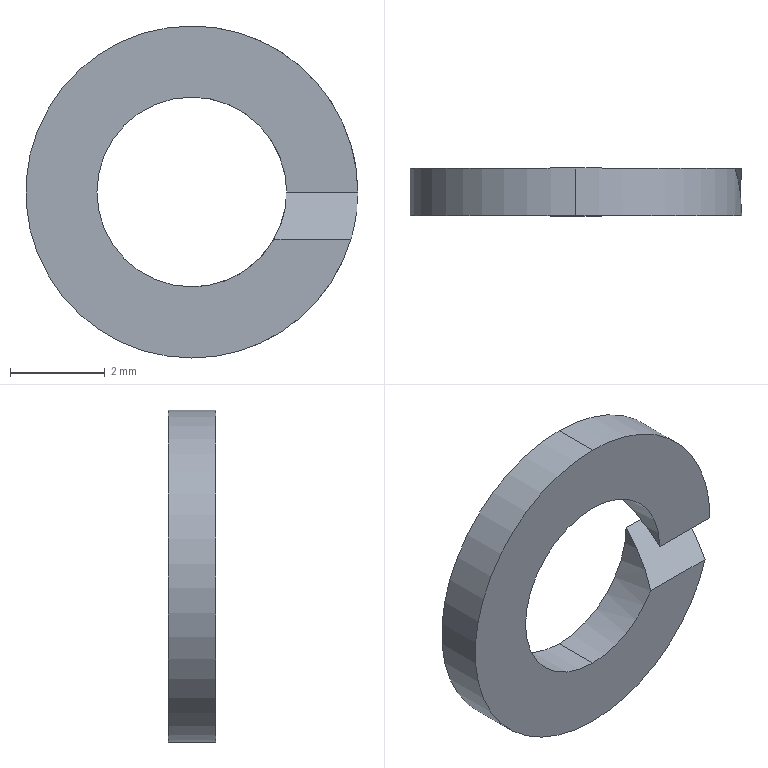Part | SolidWorks | features BaseBody 1 | 1 solid | 10 faces | box 7 x 1 x 7 mm | volume 24.399 mm3 | cylinder 6 | plane 4 | commonest cylinder face diameters 4 x3 7 x3
STEP:
#1=CARTESIAN_POINT('',(-17.5,26.,-23.5));
#2=VERTEX_POINT('',#1);
#3=CARTESIAN_POINT('',(-14.146,26.,-21.));
#4=VERTEX_POINT('',#3);
#5=CARTESIAN_POINT('',(-17.5,26.,-20.));
#6=DIRECTION('',(0.,-1.,0.));
#7=DIRECTION('',(0.,0.,1.));
#8=AXIS2_PLACEMENT_3D('',#5,#6,#7);
#9=CIRCLE('',#8,3.5);
#10=EDGE_CURVE('',#2,#4,#9,.T.);
#11=ORIENTED_EDGE('',*,*,#10,.F.);
#12=CARTESIAN_POINT('',(-17.5,27.,-23.5));
#13=VERTEX_POINT('',#12);
#14=CARTESIAN_POINT('',(-17.5,26.5,-23.5));
#15=DIRECTION('',(0.,1.,0.));
#16=VECTOR('',#15,1000.);
#17=LINE('',#14,#16);
#18=EDGE_CURVE('',#2,#13,#17,.T.);
#19=ORIENTED_EDGE('',*,*,#18,.T.);
#20=CARTESIAN_POINT('',(-14.,27.,-20.));
#21=VERTEX_POINT('',#20);
#22=CARTESIAN_POINT('',(-17.5,27.,-20.));
#23=DIRECTION('',(0.,-1.,0.));
#24=DIRECTION('',(0.,0.,1.));
#25=AXIS2_PLACEMENT_3D('',#22,#23,#24);
#26=CIRCLE('',#25,3.5);
#27=EDGE_CURVE('',#13,#21,#26,.T.);
#28=ORIENTED_EDGE('',*,*,#27,.T.);
#29=CARTESIAN_POINT('',(-14.,27.,-20.));
#30=CARTESIAN_POINT('',(-14.,26.661,-20.339));
#31=CARTESIAN_POINT('',(-14.049,26.325,-20.675));
#32=CARTESIAN_POINT('',(-14.146,26.,-21.));
#33=(BOUNDED_CURVE()B_SPLINE_CURVE(3,(#29,#30,#31,#32),.UNSPECIFIED.,.F.,.F.)B_SPLINE_CURVE_WITH_KNOTS((4,4),(1.571,1.861),.UNSPECIFIED.)CURVE()GEOMETRIC_REPRESENTATION_ITEM()RATIONAL_B_SPLINE_CURVE((1.,0.993,0.993,1.))REPRESENTATION_ITEM(''));
#34=EDGE_CURVE('',#21,#4,#33,.T.);
#35=ORIENTED_EDGE('',*,*,#34,.T.);
#36=EDGE_LOOP('',(#11,#19,#28,#35));
#37=FACE_OUTER_BOUND('',#36,.T.);
#38=CARTESIAN_POINT('',(-17.5,26.5,-20.));
#39=DIRECTION('',(0.,1.,0.));
#40=DIRECTION('',(0.,0.,1.));
#41=AXIS2_PLACEMENT_3D('',#38,#39,#40);
#42=CYLINDRICAL_SURFACE('',#41,3.5);
#43=ADVANCED_FACE('',(#37),#42,.T.);
#44=ORIENTED_EDGE('',*,*,#18,.F.);
#45=CARTESIAN_POINT('',(-17.5,26.,-16.5));
#46=VERTEX_POINT('',#45);
#47=CARTESIAN_POINT('',(-17.5,26.,-20.));
#48=DIRECTION('',(0.,-1.,0.));
#49=DIRECTION('',(0.,0.,1.));
#50=AXIS2_PLACEMENT_3D('',#47,#48,#49);
#51=CIRCLE('',#50,3.5);
#52=EDGE_CURVE('',#46,#2,#51,.T.);
#53=ORIENTED_EDGE('',*,*,#52,.F.);
#54=CARTESIAN_POINT('',(-17.5,27.,-16.5));
#55=VERTEX_POINT('',#54);
#56=CARTESIAN_POINT('',(-17.5,26.5,-16.5));
#57=DIRECTION('',(0.,1.,0.));
#58=VECTOR('',#57,1000.);
#59=LINE('',#56,#58);
#60=EDGE_CURVE('',#46,#55,#59,.T.);
#61=ORIENTED_EDGE('',*,*,#60,.T.);
#62=CARTESIAN_POINT('',(-17.5,27.,-20.));
#63=DIRECTION('',(0.,-1.,0.));
#64=DIRECTION('',(0.,0.,1.));
#65=AXIS2_PLACEMENT_3D('',#62,#63,#64);
#66=CIRCLE('',#65,3.5);
#67=EDGE_CURVE('',#55,#13,#66,.T.);
#68=ORIENTED_EDGE('',*,*,#67,.T.);
#69=EDGE_LOOP('',(#44,#53,#61,#68));
#70=FACE_OUTER_BOUND('',#69,.T.);
#71=CARTESIAN_POINT('',(-17.5,26.5,-20.));
#72=DIRECTION('',(0.,1.,0.));
#73=DIRECTION('',(0.,0.,1.));
#74=AXIS2_PLACEMENT_3D('',#71,#72,#73);
#75=CYLINDRICAL_SURFACE('',#74,3.5);
#76=ADVANCED_FACE('',(#70),#75,.T.);
#77=CARTESIAN_POINT('',(-17.5,26.,-22.));
#78=VERTEX_POINT('',#77);
#79=CARTESIAN_POINT('',(-17.5,26.,-18.));
#80=VERTEX_POINT('',#79);
#81=CARTESIAN_POINT('',(-17.5,26.,-20.));
#82=DIRECTION('',(0.,1.,0.));
#83=DIRECTION('',(0.,0.,1.));
#84=AXIS2_PLACEMENT_3D('',#81,#82,#83);
#85=CIRCLE('',#84,2.);
#86=EDGE_CURVE('',#78,#80,#85,.T.);
#87=ORIENTED_EDGE('',*,*,#86,.F.);
#88=CARTESIAN_POINT('',(-17.5,27.,-22.));
#89=VERTEX_POINT('',#88);
#90=CARTESIAN_POINT('',(-17.5,26.5,-22.));
#91=DIRECTION('',(0.,1.,0.));
#92=VECTOR('',#91,1000.);
#93=LINE('',#90,#92);
#94=EDGE_CURVE('',#78,#89,#93,.T.);
#95=ORIENTED_EDGE('',*,*,#94,.T.);
#96=CARTESIAN_POINT('',(-17.5,27.,-18.));
#97=VERTEX_POINT('',#96);
#98=CARTESIAN_POINT('',(-17.5,27.,-20.));
#99=DIRECTION('',(0.,-1.,0.));
#100=DIRECTION('',(0.,0.,1.));
#101=AXIS2_PLACEMENT_3D('',#98,#99,#100);
#102=CIRCLE('',#101,2.);
#103=EDGE_CURVE('',#97,#89,#102,.T.);
#104=ORIENTED_EDGE('',*,*,#103,.F.);
#105=CARTESIAN_POINT('',(-17.5,26.5,-18.));
#106=DIRECTION('',(0.,1.,0.));
#107=VECTOR('',#106,1000.);
#108=LINE('',#105,#107);
#109=EDGE_CURVE('',#80,#97,#108,.T.);
#110=ORIENTED_EDGE('',*,*,#109,.F.);
#111=EDGE_LOOP('',(#87,#95,#104,#110));
#112=FACE_OUTER_BOUND('',#111,.T.);
#113=CARTESIAN_POINT('',(-17.5,26.5,-20.));
#114=DIRECTION('',(0.,1.,0.));
#115=DIRECTION('',(0.,0.,1.));
#116=AXIS2_PLACEMENT_3D('',#113,#114,#115);
#117=CYLINDRICAL_SURFACE('',#116,2.);
#118=ADVANCED_FACE('',(#112),#117,.F.);
#119=CARTESIAN_POINT('',(-15.5,26.,-20.));
#120=VERTEX_POINT('',#119);
#121=CARTESIAN_POINT('',(-17.5,26.,-20.));
#122=DIRECTION('',(0.,1.,0.));
#123=DIRECTION('',(0.,0.,1.));
#124=AXIS2_PLACEMENT_3D('',#121,#122,#123);
#125=CIRCLE('',#124,2.);
#126=EDGE_CURVE('',#80,#120,#125,.T.);
#127=ORIENTED_EDGE('',*,*,#126,.F.);
#128=ORIENTED_EDGE('',*,*,#109,.T.);
#129=CARTESIAN_POINT('',(-15.768,27.,-19.));
#130=VERTEX_POINT('',#129);
#131=CARTESIAN_POINT('',(-17.5,27.,-20.));
#132=DIRECTION('',(0.,-1.,0.));
#133=DIRECTION('',(0.,0.,1.));
#134=AXIS2_PLACEMENT_3D('',#131,#132,#133);
#135=CIRCLE('',#134,2.);
#136=EDGE_CURVE('',#130,#97,#135,.T.);
#137=ORIENTED_EDGE('',*,*,#136,.F.);
#138=CARTESIAN_POINT('',(-15.768,27.,-19.));
#139=CARTESIAN_POINT('',(-15.591,26.694,-19.306));
#140=CARTESIAN_POINT('',(-15.5,26.353,-19.647));
#141=CARTESIAN_POINT('',(-15.5,26.,-20.));
#142=(BOUNDED_CURVE()B_SPLINE_CURVE(3,(#138,#139,#140,#141),.UNSPECIFIED.,.F.,.F.)B_SPLINE_CURVE_WITH_KNOTS((4,4),(1.047,1.571),.UNSPECIFIED.)CURVE()GEOMETRIC_REPRESENTATION_ITEM()RATIONAL_B_SPLINE_CURVE((1.,0.9773,0.9773,1.))REPRESENTATION_ITEM(''));
#143=EDGE_CURVE('',#130,#120,#142,.T.);
#144=ORIENTED_EDGE('',*,*,#143,.T.);
#145=EDGE_LOOP('',(#127,#128,#137,#144));
#146=FACE_OUTER_BOUND('',#145,.T.);
#147=CARTESIAN_POINT('',(-17.5,26.5,-20.));
#148=DIRECTION('',(0.,1.,0.));
#149=DIRECTION('',(0.,0.,1.));
#150=AXIS2_PLACEMENT_3D('',#147,#148,#149);
#151=CYLINDRICAL_SURFACE('',#150,2.);
#152=ADVANCED_FACE('',(#146),#151,.F.);
#153=CARTESIAN_POINT('',(-14.146,27.,-19.));
#154=VERTEX_POINT('',#153);
#155=CARTESIAN_POINT('',(-17.5,27.,-19.));
#156=DIRECTION('',(-1.,0.,0.));
#157=VECTOR('',#156,1000.);
#158=LINE('',#155,#157);
#159=EDGE_CURVE('',#154,#130,#158,.T.);
#160=ORIENTED_EDGE('',*,*,#159,.T.);
#161=ORIENTED_EDGE('',*,*,#136,.T.);
#162=ORIENTED_EDGE('',*,*,#103,.T.);
#163=CARTESIAN_POINT('',(-15.5,27.,-20.));
#164=VERTEX_POINT('',#163);
#165=CARTESIAN_POINT('',(-17.5,27.,-20.));
#166=DIRECTION('',(0.,-1.,0.));
#167=DIRECTION('',(0.,0.,1.));
#168=AXIS2_PLACEMENT_3D('',#165,#166,#167);
#169=CIRCLE('',#168,2.);
#170=EDGE_CURVE('',#89,#164,#169,.T.);
#171=ORIENTED_EDGE('',*,*,#170,.T.);
#172=CARTESIAN_POINT('',(-17.5,27.,-20.));
#173=DIRECTION('',(1.,0.,0.));
#174=VECTOR('',#173,1000.);
#175=LINE('',#172,#174);
#176=EDGE_CURVE('',#164,#21,#175,.T.);
#177=ORIENTED_EDGE('',*,*,#176,.T.);
#178=ORIENTED_EDGE('',*,*,#27,.F.);
#179=ORIENTED_EDGE('',*,*,#67,.F.);
#180=CARTESIAN_POINT('',(-17.5,27.,-20.));
#181=DIRECTION('',(0.,-1.,0.));
#182=DIRECTION('',(0.,0.,1.));
#183=AXIS2_PLACEMENT_3D('',#180,#181,#182);
#184=CIRCLE('',#183,3.5);
#185=EDGE_CURVE('',#154,#55,#184,.T.);
#186=ORIENTED_EDGE('',*,*,#185,.F.);
#187=EDGE_LOOP('',(#160,#161,#162,#171,#177,#178,#179,#186));
#188=FACE_OUTER_BOUND('',#187,.T.);
#189=CARTESIAN_POINT('',(-17.5,27.,-17.25));
#190=DIRECTION('',(0.,1.,0.));
#191=DIRECTION('',(1.,0.,0.));
#192=AXIS2_PLACEMENT_3D('',#189,#190,#191);
#193=PLANE('',#192);
#194=ADVANCED_FACE('',(#188),#193,.T.);
#195=CARTESIAN_POINT('',(-15.768,26.,-21.));
#196=VERTEX_POINT('',#195);
#197=CARTESIAN_POINT('',(-17.5,26.,-21.));
#198=DIRECTION('',(-1.,0.,0.));
#199=VECTOR('',#198,1000.);
#200=LINE('',#197,#199);
#201=EDGE_CURVE('',#4,#196,#200,.T.);
#202=ORIENTED_EDGE('',*,*,#201,.F.);
#203=ORIENTED_EDGE('',*,*,#34,.F.);
#204=ORIENTED_EDGE('',*,*,#176,.F.);
#205=CARTESIAN_POINT('',(-15.5,27.,-20.));
#206=CARTESIAN_POINT('',(-15.5,26.647,-20.353));
#207=CARTESIAN_POINT('',(-15.591,26.306,-20.694));
#208=CARTESIAN_POINT('',(-15.768,26.,-21.));
#209=(BOUNDED_CURVE()B_SPLINE_CURVE(3,(#205,#206,#207,#208),.UNSPECIFIED.,.F.,.F.)B_SPLINE_CURVE_WITH_KNOTS((4,4),(1.571,2.094),.UNSPECIFIED.)CURVE()GEOMETRIC_REPRESENTATION_ITEM()RATIONAL_B_SPLINE_CURVE((1.,0.9773,0.9773,1.))REPRESENTATION_ITEM(''));
#210=EDGE_CURVE('',#164,#196,#209,.T.);
#211=ORIENTED_EDGE('',*,*,#210,.T.);
#212=EDGE_LOOP('',(#202,#203,#204,#211));
#213=FACE_OUTER_BOUND('',#212,.T.);
#214=CARTESIAN_POINT('',(-17.5,27.,-20.));
#215=DIRECTION('',(0.,0.7071,-0.7071));
#216=DIRECTION('',(-1.,0.,0.));
#217=AXIS2_PLACEMENT_3D('',#214,#215,#216);
#218=PLANE('',#217);
#219=ADVANCED_FACE('',(#213),#218,.F.);
#220=ORIENTED_EDGE('',*,*,#159,.F.);
#221=CARTESIAN_POINT('',(-14.,26.,-20.));
#222=VERTEX_POINT('',#221);
#223=CARTESIAN_POINT('',(-14.,26.,-20.));
#224=CARTESIAN_POINT('',(-14.,26.339,-19.661));
#225=CARTESIAN_POINT('',(-14.049,26.675,-19.325));
#226=CARTESIAN_POINT('',(-14.146,27.,-19.));
#227=(BOUNDED_CURVE()B_SPLINE_CURVE(3,(#223,#224,#225,#226),.UNSPECIFIED.,.F.,.T.)B_SPLINE_CURVE_WITH_KNOTS((4,4),(4.712,5.002),.UNSPECIFIED.)CURVE()GEOMETRIC_REPRESENTATION_ITEM()RATIONAL_B_SPLINE_CURVE((1.,0.993,0.993,1.))REPRESENTATION_ITEM(''));
#228=EDGE_CURVE('',#222,#154,#227,.T.);
#229=ORIENTED_EDGE('',*,*,#228,.F.);
#230=CARTESIAN_POINT('',(-17.5,26.,-20.));
#231=DIRECTION('',(1.,0.,0.));
#232=VECTOR('',#231,1000.);
#233=LINE('',#230,#232);
#234=EDGE_CURVE('',#120,#222,#233,.T.);
#235=ORIENTED_EDGE('',*,*,#234,.F.);
#236=ORIENTED_EDGE('',*,*,#143,.F.);
#237=EDGE_LOOP('',(#220,#229,#235,#236));
#238=FACE_OUTER_BOUND('',#237,.T.);
#239=CARTESIAN_POINT('',(-17.5,26.,-20.));
#240=DIRECTION('',(0.,-0.7071,0.7071));
#241=DIRECTION('',(-1.,0.,0.));
#242=AXIS2_PLACEMENT_3D('',#239,#240,#241);
#243=PLANE('',#242);
#244=ADVANCED_FACE('',(#238),#243,.F.);
#245=ORIENTED_EDGE('',*,*,#234,.T.);
#246=CARTESIAN_POINT('',(-17.5,26.,-20.));
#247=DIRECTION('',(0.,-1.,0.));
#248=DIRECTION('',(0.,0.,1.));
#249=AXIS2_PLACEMENT_3D('',#246,#247,#248);
#250=CIRCLE('',#249,3.5);
#251=EDGE_CURVE('',#222,#46,#250,.T.);
#252=ORIENTED_EDGE('',*,*,#251,.T.);
#253=ORIENTED_EDGE('',*,*,#52,.T.);
#254=ORIENTED_EDGE('',*,*,#10,.T.);
#255=ORIENTED_EDGE('',*,*,#201,.T.);
#256=CARTESIAN_POINT('',(-17.5,26.,-20.));
#257=DIRECTION('',(0.,1.,0.));
#258=DIRECTION('',(0.,0.,1.));
#259=AXIS2_PLACEMENT_3D('',#256,#257,#258);
#260=CIRCLE('',#259,2.);
#261=EDGE_CURVE('',#196,#78,#260,.T.);
#262=ORIENTED_EDGE('',*,*,#261,.T.);
#263=ORIENTED_EDGE('',*,*,#86,.T.);
#264=ORIENTED_EDGE('',*,*,#126,.T.);
#265=EDGE_LOOP('',(#245,#252,#253,#254,#255,#262,#263,#264));
#266=FACE_OUTER_BOUND('',#265,.T.);
#267=CARTESIAN_POINT('',(-17.5,26.,-17.25));
#268=DIRECTION('',(0.,-1.,0.));
#269=DIRECTION('',(0.,0.,-1.));
#270=AXIS2_PLACEMENT_3D('',#267,#268,#269);
#271=PLANE('',#270);
#272=ADVANCED_FACE('',(#266),#271,.T.);
#273=ORIENTED_EDGE('',*,*,#94,.F.);
#274=ORIENTED_EDGE('',*,*,#261,.F.);
#275=ORIENTED_EDGE('',*,*,#210,.F.);
#276=ORIENTED_EDGE('',*,*,#170,.F.);
#277=EDGE_LOOP('',(#273,#274,#275,#276));
#278=FACE_OUTER_BOUND('',#277,.T.);
#279=CARTESIAN_POINT('',(-17.5,26.5,-20.));
#280=DIRECTION('',(0.,1.,0.));
#281=DIRECTION('',(0.,0.,1.));
#282=AXIS2_PLACEMENT_3D('',#279,#280,#281);
#283=CYLINDRICAL_SURFACE('',#282,2.);
#284=ADVANCED_FACE('',(#278),#283,.F.);
#285=ORIENTED_EDGE('',*,*,#60,.F.);
#286=ORIENTED_EDGE('',*,*,#251,.F.);
#287=ORIENTED_EDGE('',*,*,#228,.T.);
#288=ORIENTED_EDGE('',*,*,#185,.T.);
#289=EDGE_LOOP('',(#285,#286,#287,#288));
#290=FACE_OUTER_BOUND('',#289,.T.);
#291=CARTESIAN_POINT('',(-17.5,26.5,-20.));
#292=DIRECTION('',(0.,1.,0.));
#293=DIRECTION('',(0.,0.,1.));
#294=AXIS2_PLACEMENT_3D('',#291,#292,#293);
#295=CYLINDRICAL_SURFACE('',#294,3.5);
#296=ADVANCED_FACE('',(#290),#295,.T.);
#297=CLOSED_SHELL('',(#43,#76,#118,#152,#194,#219,#244,#272,#284,#296));
#298=MANIFOLD_SOLID_BREP('',#297);
#299=CARTESIAN_POINT('',(0.,0.,0.));
#300=DIRECTION('',(0.,0.,1.));
#301=DIRECTION('',(1.,0.,0.));
#302=AXIS2_PLACEMENT_3D('',#299,#300,#301);
#303=(LENGTH_UNIT()NAMED_UNIT(*)SI_UNIT(.MILLI.,.METRE.));
#304=UNCERTAINTY_MEASURE_WITH_UNIT(LENGTH_MEASURE(0.00001),#303,'','');
#305=(NAMED_UNIT(*)PLANE_ANGLE_UNIT()SI_UNIT($,.RADIAN.));
#306=(NAMED_UNIT(*)SI_UNIT($,.STERADIAN.)SOLID_ANGLE_UNIT());
#307=(GEOMETRIC_REPRESENTATION_CONTEXT(3)GLOBAL_UNCERTAINTY_ASSIGNED_CONTEXT((#304))GLOBAL_UNIT_ASSIGNED_CONTEXT((#303,#305,#306))REPRESENTATION_CONTEXT('',''));
#308=ADVANCED_BREP_SHAPE_REPRESENTATION('',(#298,#302),#307);